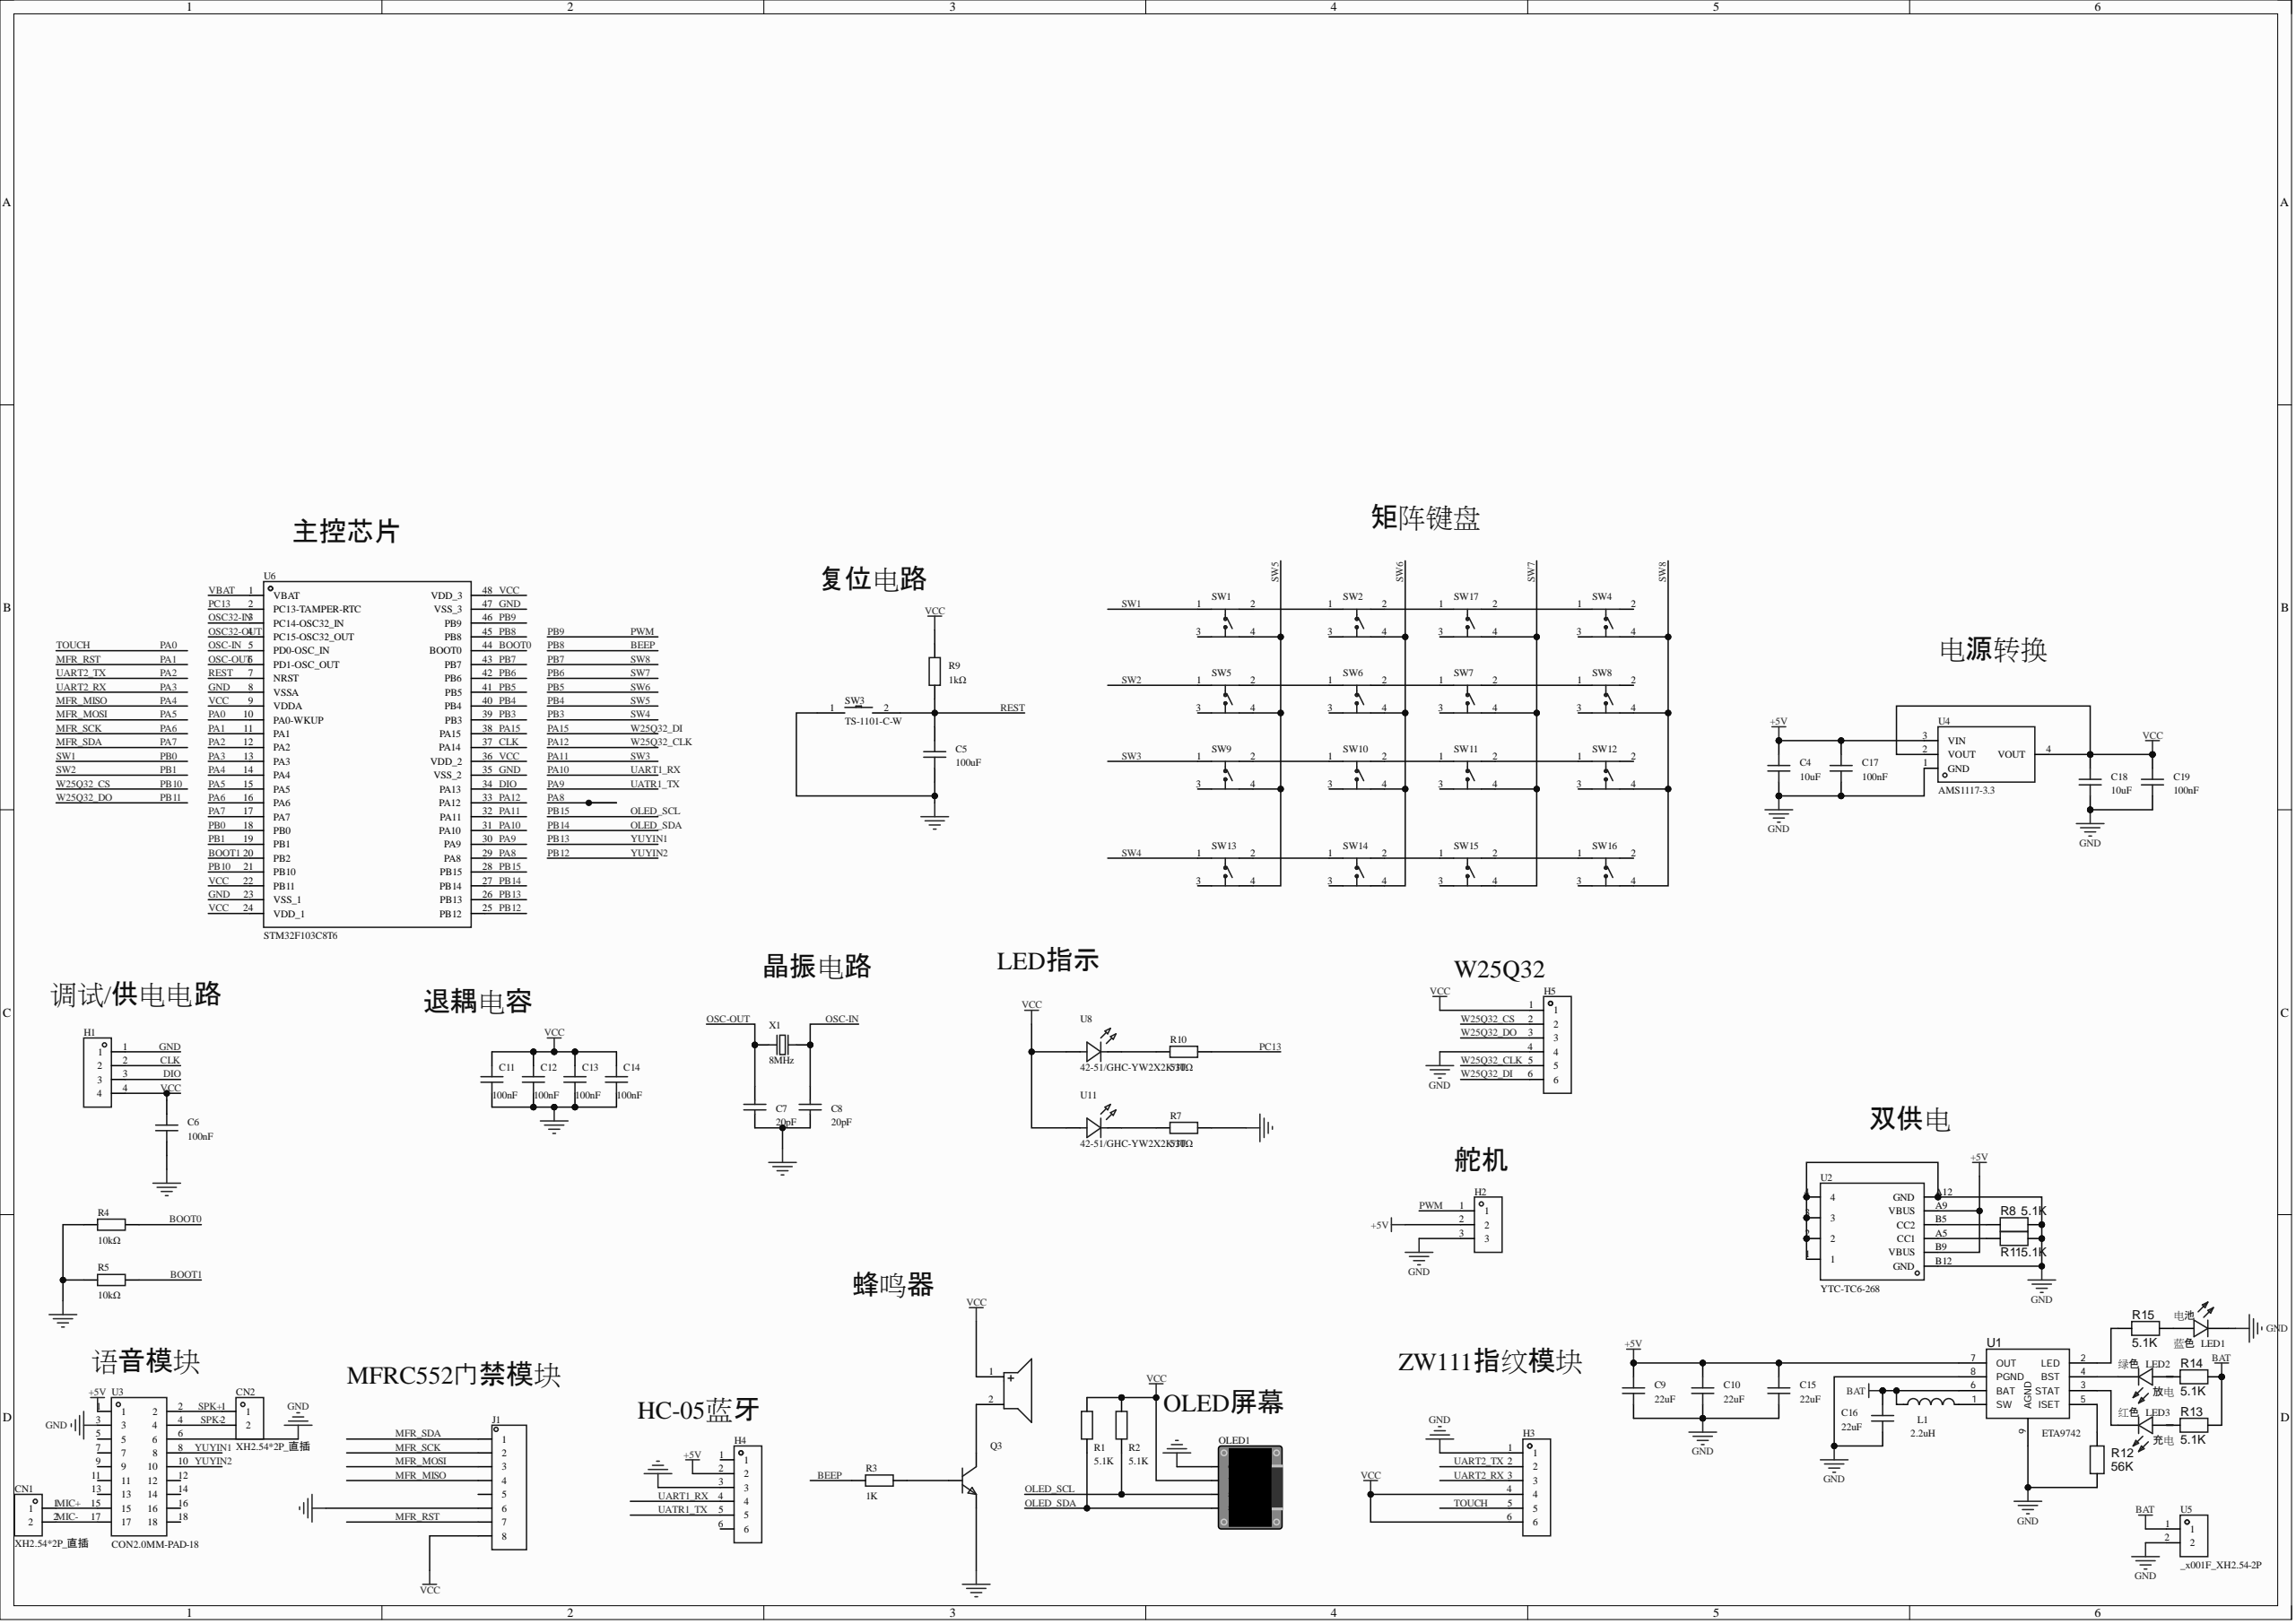Circuit board | Altium Designer | 71 parts | 69 nets
Bill of materials:
Comment,Description,Designator,Footprint,LibRef,Quantity
"2.7kHz","驱动方式:无源(外部驱动);构造类型:电磁式;频率:2.7kHz;声压(SPL):85dB;","BUZZER1","BUZ-TH_BD9.0-P4.00-D0.6-FD","QMB-09B-03","1"
"10uF","","C4, C18","C0603","CAP_0603","2"
"100uF","容值:100uF;精度:±20%;额定电压:10V;材质(温度系数):X5R;","C5","C1206","HGC1206R5107M100NSPJ","1"
"100nF","","C6, C11, C12, C13, C14, C17, C19","C0603","CGA0603X7R104K500JT, CAP_0603","7"
"20pF","容值:20pF;精度:±5%;额定电压:50V;材质(温度系数):C0G;","C7, C8","C0603","CL10C200JB8NNNC","2"
"22uF","容值:22uF;精度:±20%;额定电压:35V;材质(温度系数):X5R;","C9, C10, C15, C16","C0603","C3216X5R1V226MTJ00E","4"
"XH2.54*2P_直插","","CN1, CN2","CONN-TH_2P-P2.50-XH2.54-2P","XH2.54*2P_直插","2"
"","","H1","HDR-TH_4P-P2.54-V-F","HDR-F_2.54_1x4P","1"
"","","H2","HDR-TH_3P-P2.54-V-F","HDR-F_2.54_1x3P","1"
"","","H3, H4, H5","HDR-TH_6P-P2.54-V-F","HDR-F_2.54_1x6P","3"
"","","J1","HDR-TH_8P-P2.54-V-M","HDR-M_2.54_1x8P","1"
"2.2uH","","L1","IND-SMD_L4.4-W4.2","MWSA0402S-2R2MT","1"
"电池","","LED1","LED0603_L1.6-W0.8-RD_BLUE","NCD0603G1","1"
"放电","","LED2","LED0603_L1.6-W0.8-RD_BLUE","NCD0603G1","1"
"充电","","LED3","LED0603_L1.6-W0.8-RD_BLUE","NCD0603G1","1"
"","","OLED1","0.96OLED_4P","0.96OLED模块_4P","1"
"","","Q3","S8050_TO_92","S8050_TO_NPN","1"
"5.1K","","R1, R2","R0603","Res_0603","2"
"1K","","R3","R0603","Res_0603","1"
"10kΩ","","R4, R5","R0603","0603WAF1002T5E","2"
"510Ω","","R7, R10","R0603","0603WAF5100T5E","2"
"5.1K","","R8, R11, R13, R14, R15","R0603-NSK","NC","5"
"1kΩ","","R9","R0603","RC0603FR-071KL","1"
"56K","","R12","R0603-NSK","NC","1"
"KH-6X6X6H-TJ","电路结构:单刀单掷;按钮形状:圆形按钮;作用力:2.6N;安装方式:直插;开关长度:6mm;开关宽度:6mm;开关高度:6mm;带支架:不带支架;触点电流:50mA;额定电压:12V;工作寿命:-;","SW1, SW2, SW4, SW5, SW6, SW7, SW8, SW9, SW10, SW11, SW12, SW13, SW14, SW15, SW16, SW17","SW-TH_4P-L6.0-W6.0-P4.50-LS6.5","KH-6X6X6H-TJ","16"
"TS-1101-C-W","电路结构:单刀单掷;按钮形状:矩形按钮;作用力:260gf;安装方式:立贴;开关长度:6mm;开关宽度:3.6mm;开关高度:2.5mm;带支架:不带;触点电流:50mA;额定电压(AC):-;额定电压(DC):12V;额定功率:-;绝缘电阻:-;带灯:无;机械寿命:5万次;","SW3","SW-SMD_L6.0-W3.3-LS8.0","TS-1101-C-W","1"
"ETA9742","","U1","ESOP-8_L4.9-W3.9-P1.27-LS6.0-BL-EP","ETA9742","1"
"YTC-TC6-268","连接器类型:Type-C;公母:母座;触点数量:6;","U2","TYPE-C-SMD_YIYUAN_YTC-TC6-268","YTC-TC6-268","1"
"CON2.0MM-PAD-18","","U3","CONN-TH_18P-P2.00_C9900078766","CON2.0MM-PAD-18","1"
"AMS1117-3.3","输出类型:固定;工作电压:15V;输出电压:3.3V;输出电流:1A;电源纹波抑制比(PSRR):72dB@(120Hz);输出极性:正极;","U4","SOT-223-3_L6.5-W3.4-P2.30-LS7.0-BR","AMS1117-3.3_C6186","1"
"_x001F_XH2.54-2P","","U5","CONN-TH_2P-P2.54-V","_x001F_XH2.54-2P","1"
"STM32F103C8T6","CPU内核:ARM-M3;程序存储容量:64KB;RAM总容量:20KB;GPIO端口数量:37;工作电压范围:2V~3.6V;CPU最大主频:72MHz;程序存储器类型:FLASH;","U6","LQFP-48_L7.0-W7.0-P0.50-LS9.0-BL","STM32F103C8T6","1"
"42-51/GHC-YW2X2K/3T","发光颜色:翠绿色;正向电流:-;主波长:520nm~535nm;发光强度:2850mcd;","U8, U11","LED-SMD_L1.6-W0.8-FD_GREEN-1","42-51/GHC-YW2X2K/3T","2"
"8MHz","晶振类型:贴片晶振;频率:8MHz;常温频差:±10ppm;负载电容:12pF;频率稳定度:±20ppm;","X1","CRYSTAL-SMD_L3.2-W2.5_3225-8MHZ","X22EL89COI-111YLC-8M","1"
Netlist (Protel format):
[
BUZZER1
BUZ-TH_BD9.0-P4.00-D0.6-FD
2.7kHz



]
[
C4
C0603
10uF



]
[
C5
C1206
100uF



]
[
C6
C0603
100nF



]
[
C7
C0603
20pF



]
[
C8
C0603
20pF



]
[
C9
C0603
22uF



]
[
C10
C0603
22uF



]
[
C11
C0603
100nF



]
[
C12
C0603
100nF



]
[
C13
C0603
100nF



]
[
C14
C0603
100nF



]
[
C15
C0603
22uF



]
[
C16
C0603
22uF



]
[
C17
C0603
100nF



]
[
C18
C0603
10uF



]
[
C19
C0603
100nF



]
[
CN1
CONN-TH_2P-P2.50-XH2.54-2P
XH2.54*2P_直插



]
[
CN2
CONN-TH_2P-P2.50-XH2.54-2P
XH2.54*2P_直插



]
[
H1
HDR-TH_4P-P2.54-V-F




]
[
H2
HDR-TH_3P-P2.54-V-F




]
[
H3
HDR-TH_6P-P2.54-V-F




]
[
H4
HDR-TH_6P-P2.54-V-F




]
[
H5
HDR-TH_6P-P2.54-V-F




]
[
J1
HDR-TH_8P-P2.54-V-M




]
[
L1
IND-SMD_L4.4-W4.2
2.2uH



]
[
LED1
LED0603_L1.6-W0.8-RD_BLUE
电池



]
[
LED2
LED0603_L1.6-W0.8-RD_BLUE
放电



]
[
LED3
LED0603_L1.6-W0.8-RD_BLUE
充电



]
[
OLED1
0.96OLED_4P




]
[
Q3
S8050_TO_92




]
[
R1
R0603
5.1K



]
[
R2
R0603
5.1K



]
[
R3
R0603
1K



]
[
R4
R0603
10kΩ



]
[
R5
R0603
10kΩ



]
[
R7
R0603
510Ω



]
[
R8
R0603-NSK
5.1K



]
[
R9
R0603
1kΩ



]
[
R10
R0603
510Ω



]
[
R11
R0603-NSK
5.1K



]
[
R12
R0603-NSK
56K



]
[
R13
R0603-NSK
5.1K



]
[
R14
R0603-NSK
5.1K



]
[
R15
R0603-NSK
5.1K



]
[
SW1
SW-TH_4P-L6.0-W6.0-P4.50-LS6.5
KH-6X6X6H-TJ



]
[
SW2
SW-TH_4P-L6.0-W6.0-P4.50-LS6.5
KH-6X6X6H-TJ



]
[
SW3
SW-SMD_L6.0-W3.3-LS8.0
TS-1101-C-W



]
[
SW4
SW-TH_4P-L6.0-W6.0-P4.50-LS6.5
KH-6X6X6H-TJ



]
[
SW5
SW-TH_4P-L6.0-W6.0-P4.50-LS6.5
KH-6X6X6H-TJ



]
[
SW6
SW-TH_4P-L6.0-W6.0-P4.50-LS6.5
KH-6X6X6H-TJ



]
[
SW7
SW-TH_4P-L6.0-W6.0-P4.50-LS6.5
KH-6X6X6H-TJ



]
[
SW8
SW-TH_4P-L6.0-W6.0-P4.50-LS6.5
KH-6X6X6H-TJ



]
[
SW9
SW-TH_4P-L6.0-W6.0-P4.50-LS6.5
KH-6X6X6H-TJ



]
[
SW10
SW-TH_4P-L6.0-W6.0-P4.50-LS6.5
KH-6X6X6H-TJ



]
[
SW11
SW-TH_4P-L6.0-W6.0-P4.50-LS6.5
KH-6X6X6H-TJ



]
[
SW12
SW-TH_4P-L6.0-W6.0-P4.50-LS6.5
KH-6X6X6H-TJ



]
[
SW13
SW-TH_4P-L6.0-W6.0-P4.50-LS6.5
KH-6X6X6H-TJ



]
[
SW14
SW-TH_4P-L6.0-W6.0-P4.50-LS6.5
KH-6X6X6H-TJ



]
[
SW15
SW-TH_4P-L6.0-W6.0-P4.50-LS6.5
KH-6X6X6H-TJ



]
[
SW16
SW-TH_4P-L6.0-W6.0-P4.50-LS6.5
KH-6X6X6H-TJ



]
[
SW17
SW-TH_4P-L6.0-W6.0-P4.50-LS6.5
KH-6X6X6H-TJ



]
[
U1
ESOP-8_L4.9-W3.9-P1.27-LS6.0-BL-EP
ETA9742



]
[
U2
TYPE-C-SMD_YIYUAN_YTC-TC6-268
YTC-TC6-268



]
[
U3
CONN-TH_18P-P2.00_C9900078766
CON2.0MM-PAD-18



]
[
U4
SOT-223-3_L6.5-W3.4-P2.30-LS7.0-BR
AMS1117-3.3



]
[
U5
CONN-TH_2P-P2.54-V
_x001F_XH2.54-2P



]
[
U6
LQFP-48_L7.0-W7.0-P0.50-LS9.0-BL
STM32F103C8T6



]
[
U8
LED-SMD_L1.6-W0.8-FD_GREEN-1
42-51/GHC-YW2X2K/3T



]
[
U11
LED-SMD_L1.6-W0.8-FD_GREEN-1
42-51/GHC-YW2X2K/3T



]
[
X1
CRYSTAL-SMD_L3.2-W2.5_3225-8MHZ
8MHz



]
(
VCC
BUZZER1-1
C6-2
C11-2
C12-2
C13-2
C14-2
C18-2
C19-2
H1-4
H3-4
H3-6
H5-1
J1-8
OLED1-2
R1-2
R2-2
R9-2
U4-2
U4-4
U6-9
U6-22
U6-24
U6-36
U6-48
U8-1
U11-1
)
(
SPK-
CN2-2
U3-4
)
(
SPK+
CN2-1
U3-2
)
(
REST
C5-2
R9-1
SW3-2
U6-7
)
(
PC13
R10-2
U6-2
)
(
PB13
U3-8
U6-26
)
(
PB12
U3-10
U6-25
)
(
PB10
H5-2
U6-21
)
(
PB9
H2-1
U6-46
)
(
PB7
SW4-4
SW8-4
SW12-4
SW16-4
U6-43
)
(
PB6
SW7-4
SW11-4
SW15-4
SW17-4
U6-42
)
(
PB5
SW2-4
SW6-4
SW10-4
SW14-4
U6-41
)
(
PB4
SW1-4
SW5-4
SW9-4
SW13-4
U6-40
)
(
PB3
SW13-1
U6-39
)
(
PB1
SW5-1
U6-19
)
(
PB0
SW1-1
U6-18
)
(
PA15
H5-6
U6-38
)
(
PA12
H5-5
U6-33
)
(
PA11
SW9-1
U6-32
)
(
PA10
H4-4
U6-31
)
(
PA9
H4-5
U6-30
)
(
PA3
H3-3
U6-13
)
(
PA2
H3-2
U6-12
)
(
PA0
H3-5
U6-10
)
(
OSC-OUT
C7-2
U6-6
X1-1
)
(
OSC-IN
C8-2
U6-5
X1-2
)
(
OLED_SDA
OLED1-4
R1-1
U6-27
)
(
OLED_SCL
OLED1-3
R2-1
U6-28
)
(
NetSW15_2
SW15-2
SW16-1
)
(
NetSW14_2
SW14-2
SW15-1
)
(
NetSW13_2
SW13-2
SW14-1
)
(
NetSW11_2
SW11-2
SW12-1
)
(
NetSW10_2
SW10-2
SW11-1
)
(
NetSW9_2
SW9-2
SW10-1
)
(
NetSW7_2
SW7-2
SW8-1
)
(
NetSW6_2
SW6-2
SW7-1
)
(
NetSW5_2
SW5-2
SW6-1
)
(
NetSW4_1
SW4-1
SW17-2
)
(
NetSW2_2
SW2-2
SW17-1
)
(
NetSW1_2
SW1-2
SW2-1
)
(
NetR15_2
R15-2
U1-2
)
(
NetR12_1
R12-1
U1-5
)
(
NetR11_2
R11-2
U2-A5
)
(
NetR10_1
R10-1
U8-2
)
(
NetR8_2
R8-2
U2-B5
)
(
NetR7_1
R7-1
U11-2
)
(
NetQ3_2
Q3-2
R3-1
)
(
NetLED3_2
LED3-2
R13-2
)
(
NetLED3_1
LED3-1
U1-3
)
(
NetLED2_2
LED2-2
R14-2
)
(
NetLED2_1
LED2-1
U1-4
)
(
NetLED1_2
LED1-2
R15-1
)
(
NetL1_2
L1-2
U1-1
)
(
NetBUZZER1_2
BUZZER1-2
Q3-3
)
(
MIC-
CN1-2
U3-17
)
(
MIC+
CN1-1
U3-15
)
(
MFR_SDA
J1-1
U6-17
)
(
MFR_SCK
J1-2
U6-16
)
(
MFR_RST
J1-7
U6-11
)
(
MFR_MOSI
J1-3
U6-15
)
(
MFR_MISO
J1-4
U6-14
)
(
GND
C4-1
C5-1
C6-1
C7-1
C8-1
C9-1
C10-1
C11-1
C12-1
C13-1
C14-1
C15-1
C16-1
C17-1
C18-1
C19-1
H1-1
H2-3
H3-1
H4-3
H5-4
J1-6
LED1-1
OLED1-1
Q3-1
R4-1
R5-1
R7-2
R8-1
R11-1
R12-2
SW3-1
U1-8
U1-9
U2-1
U2-2
U2-3
U2-4
U2-A12
U2-B12
U3-3
U3-6
U4-1
U5-2
U6-8
U6-23
U6-35
U6-47
)
(
DIO
H1-3
U6-34
)
(
CLK
H1-2
U6-37
)
(
BOOT1
R5-2
U6-20
)
(
BOOT0
R4-2
U6-44
)
(
BEEP
R3-2
U6-45
)
(
BAT
C16-2
L1-1
R13-1
R14-1
U1-6
U5-1
)
(
+5V
C4-2
C9-2
C10-2
C15-2
C17-2
H2-2
H4-2
U1-7
U2-A9
U2-B9
U3-1
U4-3
)